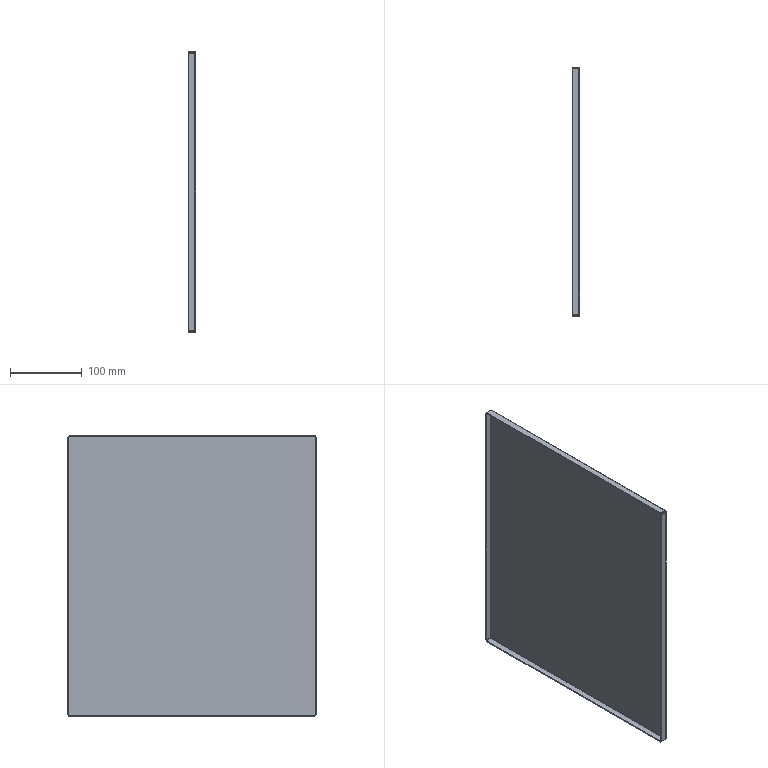Part | SolidWorks | 1 solid | 38 faces | box 10 x 346.001 x 390.001 mm | volume 220135 mm3 | plane 22 | spline 8 | cylinder 8 | commonest cylinder face diameters 0.2 x4 3.2 x4
STEP:
#1=CARTESIAN_POINT('',(-1.5,-171.4,-193.4));
#2=VERTEX_POINT('',#1);
#3=CARTESIAN_POINT('',(-1.5,171.4,-193.4));
#4=VERTEX_POINT('',#3);
#5=CARTESIAN_POINT('',(-1.5,-171.4,-193.4));
#6=DIRECTION('',(0.,1.,0.));
#7=VECTOR('',#6,1000.);
#8=LINE('',#5,#7);
#9=EDGE_CURVE('',#2,#4,#8,.T.);
#10=ORIENTED_EDGE('',*,*,#9,.F.);
#11=CARTESIAN_POINT('',(-1.5,-171.4,193.4));
#12=VERTEX_POINT('',#11);
#13=CARTESIAN_POINT('',(-1.5,-171.4,193.4));
#14=DIRECTION('',(0.,0.,-1.));
#15=VECTOR('',#14,1000.);
#16=LINE('',#13,#15);
#17=EDGE_CURVE('',#12,#2,#16,.T.);
#18=ORIENTED_EDGE('',*,*,#17,.F.);
#19=CARTESIAN_POINT('',(-1.5,171.4,193.4));
#20=VERTEX_POINT('',#19);
#21=CARTESIAN_POINT('',(-1.5,171.4,193.4));
#22=DIRECTION('',(0.,-1.,0.));
#23=VECTOR('',#22,1000.);
#24=LINE('',#21,#23);
#25=EDGE_CURVE('',#20,#12,#24,.T.);
#26=ORIENTED_EDGE('',*,*,#25,.F.);
#27=CARTESIAN_POINT('',(-1.5,171.4,-193.4));
#28=DIRECTION('',(0.,0.,1.));
#29=VECTOR('',#28,1000.);
#30=LINE('',#27,#29);
#31=EDGE_CURVE('',#4,#20,#30,.T.);
#32=ORIENTED_EDGE('',*,*,#31,.F.);
#33=EDGE_LOOP('',(#10,#18,#26,#32));
#34=FACE_OUTER_BOUND('',#33,.T.);
#35=CARTESIAN_POINT('',(-1.5,0.,0.));
#36=DIRECTION('',(1.,0.,0.));
#37=DIRECTION('',(0.,0.,-1.));
#38=AXIS2_PLACEMENT_3D('',#35,#36,#37);
#39=PLANE('',#38);
#40=ADVANCED_FACE('',(#34),#39,.F.);
#41=CARTESIAN_POINT('',(0.,-171.4,193.4));
#42=VERTEX_POINT('',#41);
#43=CARTESIAN_POINT('',(0.,-171.4,-193.4));
#44=VERTEX_POINT('',#43);
#45=CARTESIAN_POINT('',(0.,-171.4,193.4));
#46=DIRECTION('',(0.,0.,-1.));
#47=VECTOR('',#46,1000.);
#48=LINE('',#45,#47);
#49=EDGE_CURVE('',#42,#44,#48,.T.);
#50=ORIENTED_EDGE('',*,*,#49,.T.);
#51=CARTESIAN_POINT('',(0.,171.4,-193.4));
#52=VERTEX_POINT('',#51);
#53=CARTESIAN_POINT('',(0.,-171.4,-193.4));
#54=DIRECTION('',(0.,1.,0.));
#55=VECTOR('',#54,1000.);
#56=LINE('',#53,#55);
#57=EDGE_CURVE('',#44,#52,#56,.T.);
#58=ORIENTED_EDGE('',*,*,#57,.T.);
#59=CARTESIAN_POINT('',(0.,171.4,193.4));
#60=VERTEX_POINT('',#59);
#61=CARTESIAN_POINT('',(0.,171.4,-193.4));
#62=DIRECTION('',(0.,0.,1.));
#63=VECTOR('',#62,1000.);
#64=LINE('',#61,#63);
#65=EDGE_CURVE('',#52,#60,#64,.T.);
#66=ORIENTED_EDGE('',*,*,#65,.T.);
#67=CARTESIAN_POINT('',(0.,171.4,193.4));
#68=DIRECTION('',(0.,-1.,0.));
#69=VECTOR('',#68,1000.);
#70=LINE('',#67,#69);
#71=EDGE_CURVE('',#60,#42,#70,.T.);
#72=ORIENTED_EDGE('',*,*,#71,.T.);
#73=EDGE_LOOP('',(#50,#58,#66,#72));
#74=FACE_OUTER_BOUND('',#73,.T.);
#75=CARTESIAN_POINT('',(0.,0.,0.));
#76=DIRECTION('',(1.,0.,0.));
#77=DIRECTION('',(0.,0.,-1.));
#78=AXIS2_PLACEMENT_3D('',#75,#76,#77);
#79=PLANE('',#78);
#80=ADVANCED_FACE('',(#74),#79,.T.);
#81=CARTESIAN_POINT('',(-1.6,173.,192.793));
#82=VERTEX_POINT('',#81);
#83=CARTESIAN_POINT('',(-1.6,171.5,192.793));
#84=VERTEX_POINT('',#83);
#85=CARTESIAN_POINT('',(-1.6,171.5,192.793));
#86=DIRECTION('',(0.,-1.,0.));
#87=VECTOR('',#86,1000.);
#88=LINE('',#85,#87);
#89=EDGE_CURVE('',#82,#84,#88,.T.);
#90=ORIENTED_EDGE('',*,*,#89,.T.);
#91=CARTESIAN_POINT('',(-1.5,171.4,193.4));
#92=CARTESIAN_POINT('',(-1.5,171.426,193.299));
#93=CARTESIAN_POINT('',(-1.511,171.452,193.198));
#94=CARTESIAN_POINT('',(-1.548,171.489,192.995));
#95=CARTESIAN_POINT('',(-1.574,171.5,192.894));
#96=CARTESIAN_POINT('',(-1.6,171.5,192.793));
#97=B_SPLINE_CURVE_WITH_KNOTS('',3,(#91,#92,#93,#94,#95,#96),.UNSPECIFIED.,.F.,.F.,(4,2,4),(0.,0.5,1.),.UNSPECIFIED.);
#98=EDGE_CURVE('',#20,#84,#97,.T.);
#99=ORIENTED_EDGE('',*,*,#98,.F.);
#100=CARTESIAN_POINT('',(-1.5,171.4,193.4));
#101=DIRECTION('',(1.,0.,0.));
#102=VECTOR('',#101,1000.);
#103=LINE('',#100,#102);
#104=EDGE_CURVE('',#20,#60,#103,.T.);
#105=ORIENTED_EDGE('',*,*,#104,.T.);
#106=CARTESIAN_POINT('',(0.,171.4,193.4));
#107=CARTESIAN_POINT('',(0.,171.612,193.349));
#108=CARTESIAN_POINT('',(-0.04048,171.815,193.3));
#109=CARTESIAN_POINT('',(-0.2012,172.205,193.198));
#110=CARTESIAN_POINT('',(-0.3186,172.381,193.148));
#111=CARTESIAN_POINT('',(-0.5418,172.605,193.071));
#112=CARTESIAN_POINT('',(-0.6225,172.671,193.046));
#113=CARTESIAN_POINT('',(-0.7959,172.787,192.996));
#114=CARTESIAN_POINT('',(-0.8897,172.838,192.97));
#115=CARTESIAN_POINT('',(-1.18,172.958,192.894));
#116=CARTESIAN_POINT('',(-1.388,173.,192.844));
#117=CARTESIAN_POINT('',(-1.6,173.,192.793));
#118=B_SPLINE_CURVE_WITH_KNOTS('',3,(#106,#107,#108,#109,#110,#111,#112,#113,#114,#115,#116,#117),.UNSPECIFIED.,.F.,.F.,(4,2,2,2,2,4),(0.,0.0006399,0.00128,0.0016,0.00192,0.00256),.UNSPECIFIED.);
#119=EDGE_CURVE('',#60,#82,#118,.T.);
#120=ORIENTED_EDGE('',*,*,#119,.T.);
#121=EDGE_LOOP('',(#90,#99,#105,#120));
#122=FACE_OUTER_BOUND('',#121,.T.);
#123=CARTESIAN_POINT('',(0.015,171.4,193.4));
#124=CARTESIAN_POINT('',(0.015,171.611,193.349));
#125=CARTESIAN_POINT('',(-0.02703,171.823,193.299));
#126=CARTESIAN_POINT('',(-0.1888,172.213,193.198));
#127=CARTESIAN_POINT('',(-0.3085,172.392,193.147));
#128=CARTESIAN_POINT('',(-0.6075,172.691,193.046));
#129=CARTESIAN_POINT('',(-0.7867,172.811,192.995));
#130=CARTESIAN_POINT('',(-1.177,172.973,192.894));
#131=CARTESIAN_POINT('',(-1.389,173.015,192.843));
#132=CARTESIAN_POINT('',(-1.6,173.015,192.793));
#133=CARTESIAN_POINT('',(0.,171.4,193.4));
#134=CARTESIAN_POINT('',(0.,171.609,193.349));
#135=CARTESIAN_POINT('',(-0.04164,171.819,193.299));
#136=CARTESIAN_POINT('',(-0.2019,172.206,193.198));
#137=CARTESIAN_POINT('',(-0.3205,172.383,193.147));
#138=CARTESIAN_POINT('',(-0.6167,172.679,193.046));
#139=CARTESIAN_POINT('',(-0.7942,172.798,192.995));
#140=CARTESIAN_POINT('',(-1.181,172.958,192.894));
#141=CARTESIAN_POINT('',(-1.391,173.,192.843));
#142=CARTESIAN_POINT('',(-1.6,173.,192.793));
#143=CARTESIAN_POINT('',(-1.5,171.4,193.4));
#144=CARTESIAN_POINT('',(-1.5,171.413,193.349));
#145=CARTESIAN_POINT('',(-1.503,171.426,193.299));
#146=CARTESIAN_POINT('',(-1.513,171.45,193.198));
#147=CARTESIAN_POINT('',(-1.52,171.461,193.147));
#148=CARTESIAN_POINT('',(-1.539,171.48,193.046));
#149=CARTESIAN_POINT('',(-1.55,171.487,192.995));
#150=CARTESIAN_POINT('',(-1.574,171.497,192.894));
#151=CARTESIAN_POINT('',(-1.587,171.5,192.843));
#152=CARTESIAN_POINT('',(-1.6,171.5,192.793));
#153=B_SPLINE_SURFACE_WITH_KNOTS('',1,3,((#123,#124,#125,#126,#127,#128,#129,#130,#131,#132),(#133,#134,#135,#136,#137,#138,#139,#140,#141,#142),(#143,#144,#145,#146,#147,#148,#149,#150,#151,#152)),.UNSPECIFIED.,.F.,.F.,.F.,(2,1,2),(4,2,2,2,4),(-0.01,0.,1.),(0.,0.25,0.5,0.75,1.),.UNSPECIFIED.);
#154=ADVANCED_FACE('',(#122),#153,.F.);
#155=CARTESIAN_POINT('',(-1.6,171.5,-192.793));
#156=VERTEX_POINT('',#155);
#157=CARTESIAN_POINT('',(-1.6,171.5,-192.793));
#158=CARTESIAN_POINT('',(-1.574,171.5,-192.894));
#159=CARTESIAN_POINT('',(-1.548,171.489,-192.995));
#160=CARTESIAN_POINT('',(-1.511,171.452,-193.198));
#161=CARTESIAN_POINT('',(-1.5,171.426,-193.299));
#162=CARTESIAN_POINT('',(-1.5,171.4,-193.4));
#163=B_SPLINE_CURVE_WITH_KNOTS('',3,(#157,#158,#159,#160,#161,#162),.UNSPECIFIED.,.F.,.F.,(4,2,4),(0.,0.5,1.),.UNSPECIFIED.);
#164=EDGE_CURVE('',#156,#4,#163,.T.);
#165=ORIENTED_EDGE('',*,*,#164,.F.);
#166=CARTESIAN_POINT('',(-1.6,173.,-192.793));
#167=VERTEX_POINT('',#166);
#168=CARTESIAN_POINT('',(-1.6,171.5,-192.793));
#169=DIRECTION('',(0.,-1.,0.));
#170=VECTOR('',#169,1000.);
#171=LINE('',#168,#170);
#172=EDGE_CURVE('',#167,#156,#171,.T.);
#173=ORIENTED_EDGE('',*,*,#172,.F.);
#174=CARTESIAN_POINT('',(-1.6,173.,-192.793));
#175=CARTESIAN_POINT('',(-1.388,173.,-192.844));
#176=CARTESIAN_POINT('',(-1.185,172.96,-192.893));
#177=CARTESIAN_POINT('',(-0.7952,172.799,-192.995));
#178=CARTESIAN_POINT('',(-0.619,172.681,-193.045));
#179=CARTESIAN_POINT('',(-0.3953,172.458,-193.121));
#180=CARTESIAN_POINT('',(-0.329,172.378,-193.147));
#181=CARTESIAN_POINT('',(-0.2128,172.204,-193.197));
#182=CARTESIAN_POINT('',(-0.1625,172.11,-193.223));
#183=CARTESIAN_POINT('',(-0.04195,171.82,-193.299));
#184=CARTESIAN_POINT('',(0.,171.612,-193.349));
#185=CARTESIAN_POINT('',(0.,171.4,-193.4));
#186=B_SPLINE_CURVE_WITH_KNOTS('',3,(#174,#175,#176,#177,#178,#179,#180,#181,#182,#183,#184,#185),.UNSPECIFIED.,.F.,.F.,(4,2,2,2,2,4),(0.,0.0006399,0.00128,0.0016,0.00192,0.00256),.UNSPECIFIED.);
#187=EDGE_CURVE('',#167,#52,#186,.T.);
#188=ORIENTED_EDGE('',*,*,#187,.T.);
#189=CARTESIAN_POINT('',(-1.5,171.4,-193.4));
#190=DIRECTION('',(1.,0.,0.));
#191=VECTOR('',#190,1000.);
#192=LINE('',#189,#191);
#193=EDGE_CURVE('',#4,#52,#192,.T.);
#194=ORIENTED_EDGE('',*,*,#193,.F.);
#195=EDGE_LOOP('',(#165,#173,#188,#194));
#196=FACE_OUTER_BOUND('',#195,.T.);
#197=CARTESIAN_POINT('',(-1.6,173.015,-192.793));
#198=CARTESIAN_POINT('',(-1.389,173.015,-192.843));
#199=CARTESIAN_POINT('',(-1.177,172.973,-192.894));
#200=CARTESIAN_POINT('',(-0.7867,172.811,-192.995));
#201=CARTESIAN_POINT('',(-0.6075,172.691,-193.046));
#202=CARTESIAN_POINT('',(-0.3085,172.392,-193.147));
#203=CARTESIAN_POINT('',(-0.1888,172.213,-193.198));
#204=CARTESIAN_POINT('',(-0.02703,171.823,-193.299));
#205=CARTESIAN_POINT('',(0.015,171.611,-193.349));
#206=CARTESIAN_POINT('',(0.015,171.4,-193.4));
#207=CARTESIAN_POINT('',(-1.6,173.,-192.793));
#208=CARTESIAN_POINT('',(-1.391,173.,-192.843));
#209=CARTESIAN_POINT('',(-1.181,172.958,-192.894));
#210=CARTESIAN_POINT('',(-0.7942,172.798,-192.995));
#211=CARTESIAN_POINT('',(-0.6167,172.679,-193.046));
#212=CARTESIAN_POINT('',(-0.3205,172.383,-193.147));
#213=CARTESIAN_POINT('',(-0.2019,172.206,-193.198));
#214=CARTESIAN_POINT('',(-0.04164,171.819,-193.299));
#215=CARTESIAN_POINT('',(0.,171.609,-193.349));
#216=CARTESIAN_POINT('',(0.,171.4,-193.4));
#217=CARTESIAN_POINT('',(-1.6,171.5,-192.793));
#218=CARTESIAN_POINT('',(-1.587,171.5,-192.843));
#219=CARTESIAN_POINT('',(-1.574,171.497,-192.894));
#220=CARTESIAN_POINT('',(-1.55,171.487,-192.995));
#221=CARTESIAN_POINT('',(-1.539,171.48,-193.046));
#222=CARTESIAN_POINT('',(-1.52,171.461,-193.147));
#223=CARTESIAN_POINT('',(-1.513,171.45,-193.198));
#224=CARTESIAN_POINT('',(-1.503,171.426,-193.299));
#225=CARTESIAN_POINT('',(-1.5,171.413,-193.349));
#226=CARTESIAN_POINT('',(-1.5,171.4,-193.4));
#227=B_SPLINE_SURFACE_WITH_KNOTS('',1,3,((#197,#198,#199,#200,#201,#202,#203,#204,#205,#206),(#207,#208,#209,#210,#211,#212,#213,#214,#215,#216),(#217,#218,#219,#220,#221,#222,#223,#224,#225,#226)),.UNSPECIFIED.,.F.,.F.,.F.,(2,1,2),(4,2,2,2,4),(-0.01,0.,1.),(0.,0.25,0.5,0.75,1.),.UNSPECIFIED.);
#228=ADVANCED_FACE('',(#196),#227,.F.);
#229=ORIENTED_EDGE('',*,*,#65,.F.);
#230=ORIENTED_EDGE('',*,*,#187,.F.);
#231=CARTESIAN_POINT('',(-1.6,173.,0.));
#232=DIRECTION('',(0.,0.,-1.));
#233=VECTOR('',#232,1000.);
#234=LINE('',#231,#233);
#235=EDGE_CURVE('',#82,#167,#234,.T.);
#236=ORIENTED_EDGE('',*,*,#235,.F.);
#237=ORIENTED_EDGE('',*,*,#119,.F.);
#238=EDGE_LOOP('',(#229,#230,#236,#237));
#239=FACE_OUTER_BOUND('',#238,.T.);
#240=CARTESIAN_POINT('',(-1.6,171.4,-193.4));
#241=DIRECTION('',(0.,0.,-1.));
#242=DIRECTION('',(0.,1.,0.));
#243=AXIS2_PLACEMENT_3D('',#240,#241,#242);
#244=CYLINDRICAL_SURFACE('',#243,1.6);
#245=ADVANCED_FACE('',(#239),#244,.T.);
#246=ORIENTED_EDGE('',*,*,#31,.T.);
#247=ORIENTED_EDGE('',*,*,#98,.T.);
#248=CARTESIAN_POINT('',(-1.6,171.5,195.));
#249=DIRECTION('',(0.,0.,-1.));
#250=VECTOR('',#249,1000.);
#251=LINE('',#248,#250);
#252=EDGE_CURVE('',#84,#156,#251,.T.);
#253=ORIENTED_EDGE('',*,*,#252,.T.);
#254=ORIENTED_EDGE('',*,*,#164,.T.);
#255=EDGE_LOOP('',(#246,#247,#253,#254));
#256=FACE_OUTER_BOUND('',#255,.T.);
#257=CARTESIAN_POINT('',(-1.6,171.4,-193.4));
#258=DIRECTION('',(0.,0.,-1.));
#259=DIRECTION('',(0.,1.,0.));
#260=AXIS2_PLACEMENT_3D('',#257,#258,#259);
#261=CYLINDRICAL_SURFACE('',#260,0.1);
#262=ADVANCED_FACE('',(#256),#261,.F.);
#263=CARTESIAN_POINT('',(-10.,171.5,192.793));
#264=VERTEX_POINT('',#263);
#265=CARTESIAN_POINT('',(-10.,173.,192.793));
#266=VERTEX_POINT('',#265);
#267=CARTESIAN_POINT('',(-10.,173.,192.793));
#268=DIRECTION('',(0.,1.,0.));
#269=VECTOR('',#268,1000.);
#270=LINE('',#267,#269);
#271=EDGE_CURVE('',#264,#266,#270,.T.);
#272=ORIENTED_EDGE('',*,*,#271,.F.);
#273=CARTESIAN_POINT('',(0.,171.5,192.793));
#274=DIRECTION('',(-1.,0.,0.));
#275=VECTOR('',#274,1000.);
#276=LINE('',#273,#275);
#277=EDGE_CURVE('',#84,#264,#276,.T.);
#278=ORIENTED_EDGE('',*,*,#277,.F.);
#279=ORIENTED_EDGE('',*,*,#89,.F.);
#280=CARTESIAN_POINT('',(0.,173.,192.793));
#281=DIRECTION('',(1.,0.,0.));
#282=VECTOR('',#281,1000.);
#283=LINE('',#280,#282);
#284=EDGE_CURVE('',#266,#82,#283,.T.);
#285=ORIENTED_EDGE('',*,*,#284,.F.);
#286=EDGE_LOOP('',(#272,#278,#279,#285));
#287=FACE_OUTER_BOUND('',#286,.T.);
#288=CARTESIAN_POINT('',(-1.5,171.5,192.793));
#289=DIRECTION('',(0.,0.,1.));
#290=DIRECTION('',(1.,0.,0.));
#291=AXIS2_PLACEMENT_3D('',#288,#289,#290);
#292=PLANE('',#291);
#293=ADVANCED_FACE('',(#287),#292,.T.);
#294=CARTESIAN_POINT('',(-10.,173.,-192.793));
#295=VERTEX_POINT('',#294);
#296=CARTESIAN_POINT('',(-1.5,173.,-192.793));
#297=DIRECTION('',(1.,0.,0.));
#298=VECTOR('',#297,1000.);
#299=LINE('',#296,#298);
#300=EDGE_CURVE('',#295,#167,#299,.T.);
#301=ORIENTED_EDGE('',*,*,#300,.F.);
#302=CARTESIAN_POINT('',(-10.,173.,-195.));
#303=DIRECTION('',(0.,0.,-1.));
#304=VECTOR('',#303,1000.);
#305=LINE('',#302,#304);
#306=EDGE_CURVE('',#266,#295,#305,.T.);
#307=ORIENTED_EDGE('',*,*,#306,.F.);
#308=ORIENTED_EDGE('',*,*,#284,.T.);
#309=ORIENTED_EDGE('',*,*,#235,.T.);
#310=EDGE_LOOP('',(#301,#307,#308,#309));
#311=FACE_OUTER_BOUND('',#310,.T.);
#312=CARTESIAN_POINT('',(0.,173.,0.));
#313=DIRECTION('',(0.,1.,0.));
#314=DIRECTION('',(-1.,0.,0.));
#315=AXIS2_PLACEMENT_3D('',#312,#313,#314);
#316=PLANE('',#315);
#317=ADVANCED_FACE('',(#311),#316,.T.);
#318=CARTESIAN_POINT('',(-10.,171.5,-192.793));
#319=VERTEX_POINT('',#318);
#320=CARTESIAN_POINT('',(-10.,171.5,0.));
#321=DIRECTION('',(0.,0.,-1.));
#322=VECTOR('',#321,1000.);
#323=LINE('',#320,#322);
#324=EDGE_CURVE('',#264,#319,#323,.T.);
#325=ORIENTED_EDGE('',*,*,#324,.T.);
#326=CARTESIAN_POINT('',(-1.5,171.5,-192.793));
#327=DIRECTION('',(-1.,0.,0.));
#328=VECTOR('',#327,1000.);
#329=LINE('',#326,#328);
#330=EDGE_CURVE('',#156,#319,#329,.T.);
#331=ORIENTED_EDGE('',*,*,#330,.F.);
#332=ORIENTED_EDGE('',*,*,#252,.F.);
#333=ORIENTED_EDGE('',*,*,#277,.T.);
#334=EDGE_LOOP('',(#325,#331,#332,#333));
#335=FACE_OUTER_BOUND('',#334,.T.);
#336=CARTESIAN_POINT('',(0.,171.5,0.));
#337=DIRECTION('',(0.,1.,0.));
#338=DIRECTION('',(-1.,0.,0.));
#339=AXIS2_PLACEMENT_3D('',#336,#337,#338);
#340=PLANE('',#339);
#341=ADVANCED_FACE('',(#335),#340,.F.);
#342=CARTESIAN_POINT('',(-10.,171.5,-192.793));
#343=DIRECTION('',(0.,1.,0.));
#344=VECTOR('',#343,1000.);
#345=LINE('',#342,#344);
#346=EDGE_CURVE('',#319,#295,#345,.T.);
#347=ORIENTED_EDGE('',*,*,#346,.F.);
#348=ORIENTED_EDGE('',*,*,#324,.F.);
#349=ORIENTED_EDGE('',*,*,#271,.T.);
#350=ORIENTED_EDGE('',*,*,#306,.T.);
#351=EDGE_LOOP('',(#347,#348,#349,#350));
#352=FACE_OUTER_BOUND('',#351,.T.);
#353=CARTESIAN_POINT('',(-10.,173.,-195.));
#354=DIRECTION('',(-1.,0.,0.));
#355=DIRECTION('',(0.,-1.,0.));
#356=AXIS2_PLACEMENT_3D('',#353,#354,#355);
#357=PLANE('',#356);
#358=ADVANCED_FACE('',(#352),#357,.T.);
#359=ORIENTED_EDGE('',*,*,#330,.T.);
#360=ORIENTED_EDGE('',*,*,#346,.T.);
#361=ORIENTED_EDGE('',*,*,#300,.T.);
#362=ORIENTED_EDGE('',*,*,#172,.T.);
#363=EDGE_LOOP('',(#359,#360,#361,#362));
#364=FACE_OUTER_BOUND('',#363,.T.);
#365=CARTESIAN_POINT('',(-1.5,171.5,-192.793));
#366=DIRECTION('',(0.,0.,1.));
#367=DIRECTION('',(1.,0.,0.));
#368=AXIS2_PLACEMENT_3D('',#365,#366,#367);
#369=PLANE('',#368);
#370=ADVANCED_FACE('',(#364),#369,.F.);
#371=CARTESIAN_POINT('',(-1.6,-170.793,195.));
#372=VERTEX_POINT('',#371);
#373=CARTESIAN_POINT('',(-1.6,-170.793,193.5));
#374=VERTEX_POINT('',#373);
#375=CARTESIAN_POINT('',(-1.6,-170.793,193.5));
#376=DIRECTION('',(0.,0.,-1.));
#377=VECTOR('',#376,1000.);
#378=LINE('',#375,#377);
#379=EDGE_CURVE('',#372,#374,#378,.T.);
#380=ORIENTED_EDGE('',*,*,#379,.T.);
#381=CARTESIAN_POINT('',(-1.5,-171.4,193.4));
#382=CARTESIAN_POINT('',(-1.5,-171.299,193.426));
#383=CARTESIAN_POINT('',(-1.511,-171.198,193.452));
#384=CARTESIAN_POINT('',(-1.548,-170.995,193.489));
#385=CARTESIAN_POINT('',(-1.574,-170.894,193.5));
#386=CARTESIAN_POINT('',(-1.6,-170.793,193.5));
#387=B_SPLINE_CURVE_WITH_KNOTS('',3,(#381,#382,#383,#384,#385,#386),.UNSPECIFIED.,.F.,.F.,(4,2,4),(0.,0.5,1.),.UNSPECIFIED.);
#388=EDGE_CURVE('',#12,#374,#387,.T.);
#389=ORIENTED_EDGE('',*,*,#388,.F.);
#390=CARTESIAN_POINT('',(-1.5,-171.4,193.4));
#391=DIRECTION('',(1.,0.,0.));
#392=VECTOR('',#391,1000.);
#393=LINE('',#390,#392);
#394=EDGE_CURVE('',#12,#42,#393,.T.);
#395=ORIENTED_EDGE('',*,*,#394,.T.);
#396=CARTESIAN_POINT('',(0.,-171.4,193.4));
#397=CARTESIAN_POINT('',(0.,-171.349,193.612));
#398=CARTESIAN_POINT('',(-0.04048,-171.3,193.815));
#399=CARTESIAN_POINT('',(-0.2012,-171.198,194.205));
#400=CARTESIAN_POINT('',(-0.3186,-171.148,194.381));
#401=CARTESIAN_POINT('',(-0.5418,-171.071,194.605));
#402=CARTESIAN_POINT('',(-0.6225,-171.046,194.671));
#403=CARTESIAN_POINT('',(-0.7959,-170.996,194.787));
#404=CARTESIAN_POINT('',(-0.8897,-170.97,194.838));
#405=CARTESIAN_POINT('',(-1.18,-170.894,194.958));
#406=CARTESIAN_POINT('',(-1.388,-170.844,195.));
#407=CARTESIAN_POINT('',(-1.6,-170.793,195.));
#408=B_SPLINE_CURVE_WITH_KNOTS('',3,(#396,#397,#398,#399,#400,#401,#402,#403,#404,#405,#406,#407),.UNSPECIFIED.,.F.,.F.,(4,2,2,2,2,4),(0.,0.0006399,0.00128,0.0016,0.00192,0.00256),.UNSPECIFIED.);
#409=EDGE_CURVE('',#42,#372,#408,.T.);
#410=ORIENTED_EDGE('',*,*,#409,.T.);
#411=EDGE_LOOP('',(#380,#389,#395,#410));
#412=FACE_OUTER_BOUND('',#411,.T.);
#413=CARTESIAN_POINT('',(0.015,-171.4,193.4));
#414=CARTESIAN_POINT('',(0.015,-171.349,193.611));
#415=CARTESIAN_POINT('',(-0.02703,-171.299,193.823));
#416=CARTESIAN_POINT('',(-0.1888,-171.198,194.213));
#417=CARTESIAN_POINT('',(-0.3085,-171.147,194.392));
#418=CARTESIAN_POINT('',(-0.6075,-171.046,194.691));
#419=CARTESIAN_POINT('',(-0.7867,-170.995,194.811));
#420=CARTESIAN_POINT('',(-1.177,-170.894,194.973));
#421=CARTESIAN_POINT('',(-1.389,-170.843,195.015));
#422=CARTESIAN_POINT('',(-1.6,-170.793,195.015));
#423=CARTESIAN_POINT('',(0.,-171.4,193.4));
#424=CARTESIAN_POINT('',(0.,-171.349,193.609));
#425=CARTESIAN_POINT('',(-0.04164,-171.299,193.819));
#426=CARTESIAN_POINT('',(-0.2019,-171.198,194.206));
#427=CARTESIAN_POINT('',(-0.3205,-171.147,194.383));
#428=CARTESIAN_POINT('',(-0.6167,-171.046,194.679));
#429=CARTESIAN_POINT('',(-0.7942,-170.995,194.798));
#430=CARTESIAN_POINT('',(-1.181,-170.894,194.958));
#431=CARTESIAN_POINT('',(-1.391,-170.843,195.));
#432=CARTESIAN_POINT('',(-1.6,-170.793,195.));
#433=CARTESIAN_POINT('',(-1.5,-171.4,193.4));
#434=CARTESIAN_POINT('',(-1.5,-171.349,193.413));
#435=CARTESIAN_POINT('',(-1.503,-171.299,193.426));
#436=CARTESIAN_POINT('',(-1.513,-171.198,193.45));
#437=CARTESIAN_POINT('',(-1.52,-171.147,193.461));
#438=CARTESIAN_POINT('',(-1.539,-171.046,193.48));
#439=CARTESIAN_POINT('',(-1.55,-170.995,193.487));
#440=CARTESIAN_POINT('',(-1.574,-170.894,193.497));
#441=CARTESIAN_POINT('',(-1.587,-170.843,193.5));
#442=CARTESIAN_POINT('',(-1.6,-170.793,193.5));
#443=B_SPLINE_SURFACE_WITH_KNOTS('',1,3,((#413,#414,#415,#416,#417,#418,#419,#420,#421,#422),(#423,#424,#425,#426,#427,#428,#429,#430,#431,#432),(#433,#434,#435,#436,#437,#438,#439,#440,#441,#442)),.UNSPECIFIED.,.F.,.F.,.F.,(2,1,2),(4,2,2,2,4),(-0.01,0.,1.),(0.,0.25,0.5,0.75,1.),.UNSPECIFIED.);
#444=ADVANCED_FACE('',(#412),#443,.F.);
#445=CARTESIAN_POINT('',(-1.6,170.793,193.5));
#446=VERTEX_POINT('',#445);
#447=CARTESIAN_POINT('',(-1.6,170.793,193.5));
#448=CARTESIAN_POINT('',(-1.574,170.894,193.5));
#449=CARTESIAN_POINT('',(-1.548,170.995,193.489));
#450=CARTESIAN_POINT('',(-1.511,171.198,193.452));
#451=CARTESIAN_POINT('',(-1.5,171.299,193.426));
#452=CARTESIAN_POINT('',(-1.5,171.4,193.4));
#453=B_SPLINE_CURVE_WITH_KNOTS('',3,(#447,#448,#449,#450,#451,#452),.UNSPECIFIED.,.F.,.F.,(4,2,4),(0.,0.5,1.),.UNSPECIFIED.);
#454=EDGE_CURVE('',#446,#20,#453,.T.);
#455=ORIENTED_EDGE('',*,*,#454,.F.);
#456=CARTESIAN_POINT('',(-1.6,170.793,195.));
#457=VERTEX_POINT('',#456);
#458=CARTESIAN_POINT('',(-1.6,170.793,193.5));
#459=DIRECTION('',(0.,0.,-1.));
#460=VECTOR('',#459,1000.);
#461=LINE('',#458,#460);
#462=EDGE_CURVE('',#457,#446,#461,.T.);
#463=ORIENTED_EDGE('',*,*,#462,.F.);
#464=CARTESIAN_POINT('',(-1.6,170.793,195.));
#465=CARTESIAN_POINT('',(-1.388,170.844,195.));
#466=CARTESIAN_POINT('',(-1.185,170.893,194.96));
#467=CARTESIAN_POINT('',(-0.7952,170.995,194.799));
#468=CARTESIAN_POINT('',(-0.619,171.045,194.681));
#469=CARTESIAN_POINT('',(-0.3953,171.121,194.458));
#470=CARTESIAN_POINT('',(-0.329,171.147,194.378));
#471=CARTESIAN_POINT('',(-0.2128,171.197,194.204));
#472=CARTESIAN_POINT('',(-0.1625,171.223,194.11));
#473=CARTESIAN_POINT('',(-0.04195,171.299,193.82));
#474=CARTESIAN_POINT('',(0.,171.349,193.612));
#475=CARTESIAN_POINT('',(0.,171.4,193.4));
#476=B_SPLINE_CURVE_WITH_KNOTS('',3,(#464,#465,#466,#467,#468,#469,#470,#471,#472,#473,#474,#475),.UNSPECIFIED.,.F.,.F.,(4,2,2,2,2,4),(0.,0.0006399,0.00128,0.0016,0.00192,0.00256),.UNSPECIFIED.);
#477=EDGE_CURVE('',#457,#60,#476,.T.);
#478=ORIENTED_EDGE('',*,*,#477,.T.);
#479=ORIENTED_EDGE('',*,*,#104,.F.);
#480=EDGE_LOOP('',(#455,#463,#478,#479));
#481=FACE_OUTER_BOUND('',#480,.T.);
#482=CARTESIAN_POINT('',(-1.6,170.793,195.015));
#483=CARTESIAN_POINT('',(-1.389,170.843,195.015));
#484=CARTESIAN_POINT('',(-1.177,170.894,194.973));
#485=CARTESIAN_POINT('',(-0.7867,170.995,194.811));
#486=CARTESIAN_POINT('',(-0.6075,171.046,194.691));
#487=CARTESIAN_POINT('',(-0.3085,171.147,194.392));
#488=CARTESIAN_POINT('',(-0.1888,171.198,194.213));
#489=CARTESIAN_POINT('',(-0.02703,171.299,193.823));
#490=CARTESIAN_POINT('',(0.015,171.349,193.611));
#491=CARTESIAN_POINT('',(0.015,171.4,193.4));
#492=CARTESIAN_POINT('',(-1.6,170.793,195.));
#493=CARTESIAN_POINT('',(-1.391,170.843,195.));
#494=CARTESIAN_POINT('',(-1.181,170.894,194.958));
#495=CARTESIAN_POINT('',(-0.7942,170.995,194.798));
#496=CARTESIAN_POINT('',(-0.6167,171.046,194.679));
#497=CARTESIAN_POINT('',(-0.3205,171.147,194.383));
#498=CARTESIAN_POINT('',(-0.2019,171.198,194.206));
#499=CARTESIAN_POINT('',(-0.04164,171.299,193.819));
#500=CARTESIAN_POINT('',(0.,171.349,193.609));
#501=CARTESIAN_POINT('',(0.,171.4,193.4));
#502=CARTESIAN_POINT('',(-1.6,170.793,193.5));
#503=CARTESIAN_POINT('',(-1.587,170.843,193.5));
#504=CARTESIAN_POINT('',(-1.574,170.894,193.497));
#505=CARTESIAN_POINT('',(-1.55,170.995,193.487));
#506=CARTESIAN_POINT('',(-1.539,171.046,193.48));
#507=CARTESIAN_POINT('',(-1.52,171.147,193.461));
#508=CARTESIAN_POINT('',(-1.513,171.198,193.45));
#509=CARTESIAN_POINT('',(-1.503,171.299,193.426));
#510=CARTESIAN_POINT('',(-1.5,171.349,193.413));
#511=CARTESIAN_POINT('',(-1.5,171.4,193.4));
#512=B_SPLINE_SURFACE_WITH_KNOTS('',1,3,((#482,#483,#484,#485,#486,#487,#488,#489,#490,#491),(#492,#493,#494,#495,#496,#497,#498,#499,#500,#501),(#502,#503,#504,#505,#506,#507,#508,#509,#510,#511)),.UNSPECIFIED.,.F.,.F.,.F.,(2,1,2),(4,2,2,2,4),(-0.01,0.,1.),(0.,0.25,0.5,0.75,1.),.UNSPECIFIED.);
#513=ADVANCED_FACE('',(#481),#512,.F.);
#514=ORIENTED_EDGE('',*,*,#71,.F.);
#515=ORIENTED_EDGE('',*,*,#477,.F.);
#516=CARTESIAN_POINT('',(-1.6,-173.,195.));
#517=DIRECTION('',(0.,-1.,0.));
#518=VECTOR('',#517,1000.);
#519=LINE('',#516,#518);
#520=EDGE_CURVE('',#457,#372,#519,.T.);
#521=ORIENTED_EDGE('',*,*,#520,.T.);
#522=ORIENTED_EDGE('',*,*,#409,.F.);
#523=EDGE_LOOP('',(#514,#515,#521,#522));
#524=FACE_OUTER_BOUND('',#523,.T.);
#525=CARTESIAN_POINT('',(-1.6,171.4,193.4));
#526=DIRECTION('',(0.,1.,0.));
#527=DIRECTION('',(0.,0.,1.));
#528=AXIS2_PLACEMENT_3D('',#525,#526,#527);
#529=CYLINDRICAL_SURFACE('',#528,1.6);
#530=ADVANCED_FACE('',(#524),#529,.T.);
#531=ORIENTED_EDGE('',*,*,#25,.T.);
#532=ORIENTED_EDGE('',*,*,#388,.T.);
#533=CARTESIAN_POINT('',(-1.6,-173.,193.5));
#534=DIRECTION('',(0.,1.,0.));
#535=VECTOR('',#534,1000.);
#536=LINE('',#533,#535);
#537=EDGE_CURVE('',#374,#446,#536,.T.);
#538=ORIENTED_EDGE('',*,*,#537,.T.);
#539=ORIENTED_EDGE('',*,*,#454,.T.);
#540=EDGE_LOOP('',(#531,#532,#538,#539));
#541=FACE_OUTER_BOUND('',#540,.T.);
#542=CARTESIAN_POINT('',(-1.6,171.4,193.4));
#543=DIRECTION('',(0.,1.,0.));
#544=DIRECTION('',(0.,0.,1.));
#545=AXIS2_PLACEMENT_3D('',#542,#543,#544);
#546=CYLINDRICAL_SURFACE('',#545,0.1);
#547=ADVANCED_FACE('',(#541),#546,.F.);
#548=CARTESIAN_POINT('',(-10.,-170.793,193.5));
#549=VERTEX_POINT('',#548);
#550=CARTESIAN_POINT('',(-10.,-170.793,195.));
#551=VERTEX_POINT('',#550);
#552=CARTESIAN_POINT('',(-10.,-170.793,195.));
#553=DIRECTION('',(0.,0.,1.));
#554=VECTOR('',#553,1000.);
#555=LINE('',#552,#554);
#556=EDGE_CURVE('',#549,#551,#555,.T.);
#557=ORIENTED_EDGE('',*,*,#556,.F.);
#558=CARTESIAN_POINT('',(0.,-170.793,193.5));
#559=DIRECTION('',(-1.,0.,0.));
#560=VECTOR('',#559,1000.);
#561=LINE('',#558,#560);
#562=EDGE_CURVE('',#374,#549,#561,.T.);
#563=ORIENTED_EDGE('',*,*,#562,.F.);
#564=ORIENTED_EDGE('',*,*,#379,.F.);
#565=CARTESIAN_POINT('',(-1.5,-170.793,195.));
#566=DIRECTION('',(-1.,0.,0.));
#567=VECTOR('',#566,1000.);
#568=LINE('',#565,#567);
#569=EDGE_CURVE('',#372,#551,#568,.T.);
#570=ORIENTED_EDGE('',*,*,#569,.T.);
#571=EDGE_LOOP('',(#557,#563,#564,#570));
#572=FACE_OUTER_BOUND('',#571,.T.);
#573=CARTESIAN_POINT('',(-1.5,-170.793,193.5));
#574=DIRECTION('',(0.,-1.,0.));
#575=DIRECTION('',(0.,0.,-1.));
#576=AXIS2_PLACEMENT_3D('',#573,#574,#575);
#577=PLANE('',#576);
#578=ADVANCED_FACE('',(#572),#577,.T.);
#579=ORIENTED_EDGE('',*,*,#520,.F.);
#580=CARTESIAN_POINT('',(-10.,170.793,195.));
#581=VERTEX_POINT('',#580);
#582=CARTESIAN_POINT('',(0.,170.793,195.));
#583=DIRECTION('',(-1.,0.,0.));
#584=VECTOR('',#583,1000.);
#585=LINE('',#582,#584);
#586=EDGE_CURVE('',#457,#581,#585,.T.);
#587=ORIENTED_EDGE('',*,*,#586,.T.);
#588=CARTESIAN_POINT('',(-10.,-173.,195.));
#589=DIRECTION('',(0.,1.,0.));
#590=VECTOR('',#589,1000.);
#591=LINE('',#588,#590);
#592=EDGE_CURVE('',#551,#581,#591,.T.);
#593=ORIENTED_EDGE('',*,*,#592,.F.);
#594=ORIENTED_EDGE('',*,*,#569,.F.);
#595=EDGE_LOOP('',(#579,#587,#593,#594));
#596=FACE_OUTER_BOUND('',#595,.T.);
#597=CARTESIAN_POINT('',(0.,0.,195.));
#598=DIRECTION('',(0.,0.,-1.));
#599=DIRECTION('',(-1.,0.,0.));
#600=AXIS2_PLACEMENT_3D('',#597,#598,#599);
#601=PLANE('',#600);
#602=ADVANCED_FACE('',(#596),#601,.F.);
#603=CARTESIAN_POINT('',(-10.,170.793,193.5));
#604=VERTEX_POINT('',#603);
#605=CARTESIAN_POINT('',(-1.5,170.793,193.5));
#606=DIRECTION('',(-1.,0.,0.));
#607=VECTOR('',#606,1000.);
#608=LINE('',#605,#607);
#609=EDGE_CURVE('',#446,#604,#608,.T.);
#610=ORIENTED_EDGE('',*,*,#609,.F.);
#611=ORIENTED_EDGE('',*,*,#537,.F.);
#612=ORIENTED_EDGE('',*,*,#562,.T.);
#613=CARTESIAN_POINT('',(-10.,0.,193.5));
#614=DIRECTION('',(0.,1.,0.));
#615=VECTOR('',#614,1000.);
#616=LINE('',#613,#615);
#617=EDGE_CURVE('',#549,#604,#616,.T.);
#618=ORIENTED_EDGE('',*,*,#617,.T.);
#619=EDGE_LOOP('',(#610,#611,#612,#618));
#620=FACE_OUTER_BOUND('',#619,.T.);
#621=CARTESIAN_POINT('',(0.,0.,193.5));
#622=DIRECTION('',(0.,0.,-1.));
#623=DIRECTION('',(-1.,0.,0.));
#624=AXIS2_PLACEMENT_3D('',#621,#622,#623);
#625=PLANE('',#624);
#626=ADVANCED_FACE('',(#620),#625,.T.);
#627=CARTESIAN_POINT('',(-10.,170.793,193.5));
#628=DIRECTION('',(0.,0.,1.));
#629=VECTOR('',#628,1000.);
#630=LINE('',#627,#629);
#631=EDGE_CURVE('',#604,#581,#630,.T.);
#632=ORIENTED_EDGE('',*,*,#631,.F.);
#633=ORIENTED_EDGE('',*,*,#617,.F.);
#634=ORIENTED_EDGE('',*,*,#556,.T.);
#635=ORIENTED_EDGE('',*,*,#592,.T.);
#636=EDGE_LOOP('',(#632,#633,#634,#635));
#637=FACE_OUTER_BOUND('',#636,.T.);
#638=CARTESIAN_POINT('',(-10.,-173.,195.));
#639=DIRECTION('',(-1.,0.,0.));
#640=DIRECTION('',(0.,0.,1.));
#641=AXIS2_PLACEMENT_3D('',#638,#639,#640);
#642=PLANE('',#641);
#643=ADVANCED_FACE('',(#637),#642,.T.);
#644=ORIENTED_EDGE('',*,*,#609,.T.);
#645=ORIENTED_EDGE('',*,*,#631,.T.);
#646=ORIENTED_EDGE('',*,*,#586,.F.);
#647=ORIENTED_EDGE('',*,*,#462,.T.);
#648=EDGE_LOOP('',(#644,#645,#646,#647));
#649=FACE_OUTER_BOUND('',#648,.T.);
#650=CARTESIAN_POINT('',(-1.5,170.793,193.5));
#651=DIRECTION('',(0.,-1.,0.));
#652=DIRECTION('',(0.,0.,-1.));
#653=AXIS2_PLACEMENT_3D('',#650,#651,#652);
#654=PLANE('',#653);
#655=ADVANCED_FACE('',(#649),#654,.F.);
#656=CARTESIAN_POINT('',(-1.6,-173.,-192.793));
#657=VERTEX_POINT('',#656);
#658=CARTESIAN_POINT('',(-1.6,-171.5,-192.793));
#659=VERTEX_POINT('',#658);
#660=CARTESIAN_POINT('',(-1.6,-171.5,-192.793));
#661=DIRECTION('',(0.,1.,0.));
#662=VECTOR('',#661,1000.);
#663=LINE('',#660,#662);
#664=EDGE_CURVE('',#657,#659,#663,.T.);
#665=ORIENTED_EDGE('',*,*,#664,.T.);
#666=CARTESIAN_POINT('',(-1.5,-171.4,-193.4));
#667=CARTESIAN_POINT('',(-1.5,-171.426,-193.299));
#668=CARTESIAN_POINT('',(-1.511,-171.452,-193.198));
#669=CARTESIAN_POINT('',(-1.548,-171.489,-192.995));
#670=CARTESIAN_POINT('',(-1.574,-171.5,-192.894));
#671=CARTESIAN_POINT('',(-1.6,-171.5,-192.793));
#672=B_SPLINE_CURVE_WITH_KNOTS('',3,(#666,#667,#668,#669,#670,#671),.UNSPECIFIED.,.F.,.F.,(4,2,4),(0.,0.5,1.),.UNSPECIFIED.);
#673=EDGE_CURVE('',#2,#659,#672,.T.);
#674=ORIENTED_EDGE('',*,*,#673,.F.);
#675=CARTESIAN_POINT('',(-1.5,-171.4,-193.4));
#676=DIRECTION('',(1.,0.,0.));
#677=VECTOR('',#676,1000.);
#678=LINE('',#675,#677);
#679=EDGE_CURVE('',#2,#44,#678,.T.);
#680=ORIENTED_EDGE('',*,*,#679,.T.);
#681=CARTESIAN_POINT('',(0.,-171.4,-193.4));
#682=CARTESIAN_POINT('',(0.,-171.612,-193.349));
#683=CARTESIAN_POINT('',(-0.04048,-171.815,-193.3));
#684=CARTESIAN_POINT('',(-0.2012,-172.205,-193.198));
#685=CARTESIAN_POINT('',(-0.3186,-172.381,-193.148));
#686=CARTESIAN_POINT('',(-0.5418,-172.605,-193.071));
#687=CARTESIAN_POINT('',(-0.6225,-172.671,-193.046));
#688=CARTESIAN_POINT('',(-0.7959,-172.787,-192.996));
#689=CARTESIAN_POINT('',(-0.8897,-172.838,-192.97));
#690=CARTESIAN_POINT('',(-1.18,-172.958,-192.894));
#691=CARTESIAN_POINT('',(-1.388,-173.,-192.844));
#692=CARTESIAN_POINT('',(-1.6,-173.,-192.793));
#693=B_SPLINE_CURVE_WITH_KNOTS('',3,(#681,#682,#683,#684,#685,#686,#687,#688,#689,#690,#691,#692),.UNSPECIFIED.,.F.,.F.,(4,2,2,2,2,4),(0.,0.0006399,0.00128,0.0016,0.00192,0.00256),.UNSPECIFIED.);
#694=EDGE_CURVE('',#44,#657,#693,.T.);
#695=ORIENTED_EDGE('',*,*,#694,.T.);
#696=EDGE_LOOP('',(#665,#674,#680,#695));
#697=FACE_OUTER_BOUND('',#696,.T.);
#698=CARTESIAN_POINT('',(0.015,-171.4,-193.4));
#699=CARTESIAN_POINT('',(0.015,-171.611,-193.349));
#700=CARTESIAN_POINT('',(-0.02703,-171.823,-193.299));
#701=CARTESIAN_POINT('',(-0.1888,-172.213,-193.198));
#702=CARTESIAN_POINT('',(-0.3085,-172.392,-193.147));
#703=CARTESIAN_POINT('',(-0.6075,-172.691,-193.046));
#704=CARTESIAN_POINT('',(-0.7867,-172.811,-192.995));
#705=CARTESIAN_POINT('',(-1.177,-172.973,-192.894));
#706=CARTESIAN_POINT('',(-1.389,-173.015,-192.843));
#707=CARTESIAN_POINT('',(-1.6,-173.015,-192.793));
#708=CARTESIAN_POINT('',(0.,-171.4,-193.4));
#709=CARTESIAN_POINT('',(0.,-171.609,-193.349));
#710=CARTESIAN_POINT('',(-0.04164,-171.819,-193.299));
#711=CARTESIAN_POINT('',(-0.2019,-172.206,-193.198));
#712=CARTESIAN_POINT('',(-0.3205,-172.383,-193.147));
#713=CARTESIAN_POINT('',(-0.6167,-172.679,-193.046));
#714=CARTESIAN_POINT('',(-0.7942,-172.798,-192.995));
#715=CARTESIAN_POINT('',(-1.181,-172.958,-192.894));
#716=CARTESIAN_POINT('',(-1.391,-173.,-192.843));
#717=CARTESIAN_POINT('',(-1.6,-173.,-192.793));
#718=CARTESIAN_POINT('',(-1.5,-171.4,-193.4));
#719=CARTESIAN_POINT('',(-1.5,-171.413,-193.349));
#720=CARTESIAN_POINT('',(-1.503,-171.426,-193.299));
#721=CARTESIAN_POINT('',(-1.513,-171.45,-193.198));
#722=CARTESIAN_POINT('',(-1.52,-171.461,-193.147));
#723=CARTESIAN_POINT('',(-1.539,-171.48,-193.046));
#724=CARTESIAN_POINT('',(-1.55,-171.487,-192.995));
#725=CARTESIAN_POINT('',(-1.574,-171.497,-192.894));
#726=CARTESIAN_POINT('',(-1.587,-171.5,-192.843));
#727=CARTESIAN_POINT('',(-1.6,-171.5,-192.793));
#728=B_SPLINE_SURFACE_WITH_KNOTS('',1,3,((#698,#699,#700,#701,#702,#703,#704,#705,#706,#707),(#708,#709,#710,#711,#712,#713,#714,#715,#716,#717),(#718,#719,#720,#721,#722,#723,#724,#725,#726,#727)),.UNSPECIFIED.,.F.,.F.,.F.,(2,1,2),(4,2,2,2,4),(-0.01,0.,1.),(0.,0.25,0.5,0.75,1.),.UNSPECIFIED.);
#729=ADVANCED_FACE('',(#697),#728,.F.);
#730=CARTESIAN_POINT('',(-1.6,-171.5,192.793));
#731=VERTEX_POINT('',#730);
#732=CARTESIAN_POINT('',(-1.6,-171.5,192.793));
#733=CARTESIAN_POINT('',(-1.574,-171.5,192.894));
#734=CARTESIAN_POINT('',(-1.548,-171.489,192.995));
#735=CARTESIAN_POINT('',(-1.511,-171.452,193.198));
#736=CARTESIAN_POINT('',(-1.5,-171.426,193.299));
#737=CARTESIAN_POINT('',(-1.5,-171.4,193.4));
#738=B_SPLINE_CURVE_WITH_KNOTS('',3,(#732,#733,#734,#735,#736,#737),.UNSPECIFIED.,.F.,.F.,(4,2,4),(0.,0.5,1.),.UNSPECIFIED.);
#739=EDGE_CURVE('',#731,#12,#738,.T.);
#740=ORIENTED_EDGE('',*,*,#739,.F.);
#741=CARTESIAN_POINT('',(-1.6,-173.,192.793));
#742=VERTEX_POINT('',#741);
#743=CARTESIAN_POINT('',(-1.6,-171.5,192.793));
#744=DIRECTION('',(0.,1.,0.));
#745=VECTOR('',#744,1000.);
#746=LINE('',#743,#745);
#747=EDGE_CURVE('',#742,#731,#746,.T.);
#748=ORIENTED_EDGE('',*,*,#747,.F.);
#749=CARTESIAN_POINT('',(-1.6,-173.,192.793));
#750=CARTESIAN_POINT('',(-1.388,-173.,192.844));
#751=CARTESIAN_POINT('',(-1.185,-172.96,192.893));
#752=CARTESIAN_POINT('',(-0.7952,-172.799,192.995));
#753=CARTESIAN_POINT('',(-0.619,-172.681,193.045));
#754=CARTESIAN_POINT('',(-0.3953,-172.458,193.121));
#755=CARTESIAN_POINT('',(-0.329,-172.378,193.147));
#756=CARTESIAN_POINT('',(-0.2128,-172.204,193.197));
#757=CARTESIAN_POINT('',(-0.1625,-172.11,193.223));
#758=CARTESIAN_POINT('',(-0.04195,-171.82,193.299));
#759=CARTESIAN_POINT('',(0.,-171.612,193.349));
#760=CARTESIAN_POINT('',(0.,-171.4,193.4));
#761=B_SPLINE_CURVE_WITH_KNOTS('',3,(#749,#750,#751,#752,#753,#754,#755,#756,#757,#758,#759,#760),.UNSPECIFIED.,.F.,.F.,(4,2,2,2,2,4),(0.,0.0006399,0.00128,0.0016,0.00192,0.00256),.UNSPECIFIED.);
#762=EDGE_CURVE('',#742,#42,#761,.T.);
#763=ORIENTED_EDGE('',*,*,#762,.T.);
#764=ORIENTED_EDGE('',*,*,#394,.F.);
#765=EDGE_LOOP('',(#740,#748,#763,#764));
#766=FACE_OUTER_BOUND('',#765,.T.);
#767=CARTESIAN_POINT('',(-1.6,-173.015,192.793));
#768=CARTESIAN_POINT('',(-1.389,-173.015,192.843));
#769=CARTESIAN_POINT('',(-1.177,-172.973,192.894));
#770=CARTESIAN_POINT('',(-0.7867,-172.811,192.995));
#771=CARTESIAN_POINT('',(-0.6075,-172.691,193.046));
#772=CARTESIAN_POINT('',(-0.3085,-172.392,193.147));
#773=CARTESIAN_POINT('',(-0.1888,-172.213,193.198));
#774=CARTESIAN_POINT('',(-0.02703,-171.823,193.299));
#775=CARTESIAN_POINT('',(0.015,-171.611,193.349));
#776=CARTESIAN_POINT('',(0.015,-171.4,193.4));
#777=CARTESIAN_POINT('',(-1.6,-173.,192.793));
#778=CARTESIAN_POINT('',(-1.391,-173.,192.843));
#779=CARTESIAN_POINT('',(-1.181,-172.958,192.894));
#780=CARTESIAN_POINT('',(-0.7942,-172.798,192.995));
#781=CARTESIAN_POINT('',(-0.6167,-172.679,193.046));
#782=CARTESIAN_POINT('',(-0.3205,-172.383,193.147));
#783=CARTESIAN_POINT('',(-0.2019,-172.206,193.198));
#784=CARTESIAN_POINT('',(-0.04164,-171.819,193.299));
#785=CARTESIAN_POINT('',(0.,-171.609,193.349));
#786=CARTESIAN_POINT('',(0.,-171.4,193.4));
#787=CARTESIAN_POINT('',(-1.6,-171.5,192.793));
#788=CARTESIAN_POINT('',(-1.587,-171.5,192.843));
#789=CARTESIAN_POINT('',(-1.574,-171.497,192.894));
#790=CARTESIAN_POINT('',(-1.55,-171.487,192.995));
#791=CARTESIAN_POINT('',(-1.539,-171.48,193.046));
#792=CARTESIAN_POINT('',(-1.52,-171.461,193.147));
#793=CARTESIAN_POINT('',(-1.513,-171.45,193.198));
#794=CARTESIAN_POINT('',(-1.503,-171.426,193.299));
#795=CARTESIAN_POINT('',(-1.5,-171.413,193.349));
#796=CARTESIAN_POINT('',(-1.5,-171.4,193.4));
#797=B_SPLINE_SURFACE_WITH_KNOTS('',1,3,((#767,#768,#769,#770,#771,#772,#773,#774,#775,#776),(#777,#778,#779,#780,#781,#782,#783,#784,#785,#786),(#787,#788,#789,#790,#791,#792,#793,#794,#795,#796)),.UNSPECIFIED.,.F.,.F.,.F.,(2,1,2),(4,2,2,2,4),(-0.01,0.,1.),(0.,0.25,0.5,0.75,1.),.UNSPECIFIED.);
#798=ADVANCED_FACE('',(#766),#797,.F.);
#799=ORIENTED_EDGE('',*,*,#49,.F.);
#800=ORIENTED_EDGE('',*,*,#762,.F.);
#801=CARTESIAN_POINT('',(-1.6,-173.,-195.));
#802=DIRECTION('',(0.,0.,-1.));
#803=VECTOR('',#802,1000.);
#804=LINE('',#801,#803);
#805=EDGE_CURVE('',#742,#657,#804,.T.);
#806=ORIENTED_EDGE('',*,*,#805,.T.);
#807=ORIENTED_EDGE('',*,*,#694,.F.);
#808=EDGE_LOOP('',(#799,#800,#806,#807));
#809=FACE_OUTER_BOUND('',#808,.T.);
#810=CARTESIAN_POINT('',(-1.6,-171.4,193.4));
#811=DIRECTION('',(0.,0.,1.));
#812=DIRECTION('',(0.,-1.,0.));
#813=AXIS2_PLACEMENT_3D('',#810,#811,#812);
#814=CYLINDRICAL_SURFACE('',#813,1.6);
#815=ADVANCED_FACE('',(#809),#814,.T.);
#816=ORIENTED_EDGE('',*,*,#17,.T.);
#817=ORIENTED_EDGE('',*,*,#673,.T.);
#818=CARTESIAN_POINT('',(-1.6,-171.5,-195.));
#819=DIRECTION('',(0.,0.,1.));
#820=VECTOR('',#819,1000.);
#821=LINE('',#818,#820);
#822=EDGE_CURVE('',#659,#731,#821,.T.);
#823=ORIENTED_EDGE('',*,*,#822,.T.);
#824=ORIENTED_EDGE('',*,*,#739,.T.);
#825=EDGE_LOOP('',(#816,#817,#823,#824));
#826=FACE_OUTER_BOUND('',#825,.T.);
#827=CARTESIAN_POINT('',(-1.6,-171.4,193.4));
#828=DIRECTION('',(0.,0.,1.));
#829=DIRECTION('',(0.,-1.,0.));
#830=AXIS2_PLACEMENT_3D('',#827,#828,#829);
#831=CYLINDRICAL_SURFACE('',#830,0.1);
#832=ADVANCED_FACE('',(#826),#831,.F.);
#833=CARTESIAN_POINT('',(-10.,-171.5,-192.793));
#834=VERTEX_POINT('',#833);
#835=CARTESIAN_POINT('',(-10.,-173.,-192.793));
#836=VERTEX_POINT('',#835);
#837=CARTESIAN_POINT('',(-10.,-173.,-192.793));
#838=DIRECTION('',(0.,-1.,0.));
#839=VECTOR('',#838,1000.);
#840=LINE('',#837,#839);
#841=EDGE_CURVE('',#834,#836,#840,.T.);
#842=ORIENTED_EDGE('',*,*,#841,.F.);
#843=CARTESIAN_POINT('',(0.,-171.5,-192.793));
#844=DIRECTION('',(-1.,0.,0.));
#845=VECTOR('',#844,1000.);
#846=LINE('',#843,#845);
#847=EDGE_CURVE('',#659,#834,#846,.T.);
#848=ORIENTED_EDGE('',*,*,#847,.F.);
#849=ORIENTED_EDGE('',*,*,#664,.F.);
#850=CARTESIAN_POINT('',(-1.5,-173.,-192.793));
#851=DIRECTION('',(-1.,0.,0.));
#852=VECTOR('',#851,1000.);
#853=LINE('',#850,#852);
#854=EDGE_CURVE('',#657,#836,#853,.T.);
#855=ORIENTED_EDGE('',*,*,#854,.T.);
#856=EDGE_LOOP('',(#842,#848,#849,#855));
#857=FACE_OUTER_BOUND('',#856,.T.);
#858=CARTESIAN_POINT('',(-1.5,-171.5,-192.793));
#859=DIRECTION('',(0.,0.,-1.));
#860=DIRECTION('',(-1.,0.,0.));
#861=AXIS2_PLACEMENT_3D('',#858,#859,#860);
#862=PLANE('',#861);
#863=ADVANCED_FACE('',(#857),#862,.T.);
#864=ORIENTED_EDGE('',*,*,#805,.F.);
#865=CARTESIAN_POINT('',(-10.,-173.,192.793));
#866=VERTEX_POINT('',#865);
#867=CARTESIAN_POINT('',(0.,-173.,192.793));
#868=DIRECTION('',(-1.,0.,0.));
#869=VECTOR('',#868,1000.);
#870=LINE('',#867,#869);
#871=EDGE_CURVE('',#742,#866,#870,.T.);
#872=ORIENTED_EDGE('',*,*,#871,.T.);
#873=CARTESIAN_POINT('',(-10.,-173.,-195.));
#874=DIRECTION('',(0.,0.,1.));
#875=VECTOR('',#874,1000.);
#876=LINE('',#873,#875);
#877=EDGE_CURVE('',#836,#866,#876,.T.);
#878=ORIENTED_EDGE('',*,*,#877,.F.);
#879=ORIENTED_EDGE('',*,*,#854,.F.);
#880=EDGE_LOOP('',(#864,#872,#878,#879));
#881=FACE_OUTER_BOUND('',#880,.T.);
#882=CARTESIAN_POINT('',(0.,-173.,0.));
#883=DIRECTION('',(0.,1.,0.));
#884=DIRECTION('',(-1.,0.,0.));
#885=AXIS2_PLACEMENT_3D('',#882,#883,#884);
#886=PLANE('',#885);
#887=ADVANCED_FACE('',(#881),#886,.F.);
#888=CARTESIAN_POINT('',(-10.,-171.5,192.793));
#889=VERTEX_POINT('',#888);
#890=CARTESIAN_POINT('',(-1.5,-171.5,192.793));
#891=DIRECTION('',(-1.,0.,0.));
#892=VECTOR('',#891,1000.);
#893=LINE('',#890,#892);
#894=EDGE_CURVE('',#731,#889,#893,.T.);
#895=ORIENTED_EDGE('',*,*,#894,.F.);
#896=ORIENTED_EDGE('',*,*,#822,.F.);
#897=ORIENTED_EDGE('',*,*,#847,.T.);
#898=CARTESIAN_POINT('',(-10.,-171.5,0.));
#899=DIRECTION('',(0.,0.,1.));
#900=VECTOR('',#899,1000.);
#901=LINE('',#898,#900);
#902=EDGE_CURVE('',#834,#889,#901,.T.);
#903=ORIENTED_EDGE('',*,*,#902,.T.);
#904=EDGE_LOOP('',(#895,#896,#897,#903));
#905=FACE_OUTER_BOUND('',#904,.T.);
#906=CARTESIAN_POINT('',(0.,-171.5,0.));
#907=DIRECTION('',(0.,1.,0.));
#908=DIRECTION('',(-1.,0.,0.));
#909=AXIS2_PLACEMENT_3D('',#906,#907,#908);
#910=PLANE('',#909);
#911=ADVANCED_FACE('',(#905),#910,.T.);
#912=CARTESIAN_POINT('',(-10.,-171.5,192.793));
#913=DIRECTION('',(0.,-1.,0.));
#914=VECTOR('',#913,1000.);
#915=LINE('',#912,#914);
#916=EDGE_CURVE('',#889,#866,#915,.T.);
#917=ORIENTED_EDGE('',*,*,#916,.F.);
#918=ORIENTED_EDGE('',*,*,#902,.F.);
#919=ORIENTED_EDGE('',*,*,#841,.T.);
#920=ORIENTED_EDGE('',*,*,#877,.T.);
#921=EDGE_LOOP('',(#917,#918,#919,#920));
#922=FACE_OUTER_BOUND('',#921,.T.);
#923=CARTESIAN_POINT('',(-10.,-173.,-195.));
#924=DIRECTION('',(-1.,0.,0.));
#925=DIRECTION('',(0.,-1.,0.));
#926=AXIS2_PLACEMENT_3D('',#923,#924,#925);
#927=PLANE('',#926);
#928=ADVANCED_FACE('',(#922),#927,.T.);
#929=ORIENTED_EDGE('',*,*,#894,.T.);
#930=ORIENTED_EDGE('',*,*,#916,.T.);
#931=ORIENTED_EDGE('',*,*,#871,.F.);
#932=ORIENTED_EDGE('',*,*,#747,.T.);
#933=EDGE_LOOP('',(#929,#930,#931,#932));
#934=FACE_OUTER_BOUND('',#933,.T.);
#935=CARTESIAN_POINT('',(-1.5,-171.5,192.793));
#936=DIRECTION('',(0.,0.,-1.));
#937=DIRECTION('',(-1.,0.,0.));
#938=AXIS2_PLACEMENT_3D('',#935,#936,#937);
#939=PLANE('',#938);
#940=ADVANCED_FACE('',(#934),#939,.F.);
#941=CARTESIAN_POINT('',(-1.6,170.793,-195.));
#942=VERTEX_POINT('',#941);
#943=CARTESIAN_POINT('',(-1.6,170.793,-193.5));
#944=VERTEX_POINT('',#943);
#945=CARTESIAN_POINT('',(-1.6,170.793,-193.5));
#946=DIRECTION('',(0.,0.,1.));
#947=VECTOR('',#946,1000.);
#948=LINE('',#945,#947);
#949=EDGE_CURVE('',#942,#944,#948,.T.);
#950=ORIENTED_EDGE('',*,*,#949,.T.);
#951=CARTESIAN_POINT('',(-1.5,171.4,-193.4));
#952=CARTESIAN_POINT('',(-1.5,171.299,-193.426));
#953=CARTESIAN_POINT('',(-1.511,171.198,-193.452));
#954=CARTESIAN_POINT('',(-1.548,170.995,-193.489));
#955=CARTESIAN_POINT('',(-1.574,170.894,-193.5));
#956=CARTESIAN_POINT('',(-1.6,170.793,-193.5));
#957=B_SPLINE_CURVE_WITH_KNOTS('',3,(#951,#952,#953,#954,#955,#956),.UNSPECIFIED.,.F.,.F.,(4,2,4),(0.,0.5,1.),.UNSPECIFIED.);
#958=EDGE_CURVE('',#4,#944,#957,.T.);
#959=ORIENTED_EDGE('',*,*,#958,.F.);
#960=ORIENTED_EDGE('',*,*,#193,.T.);
#961=CARTESIAN_POINT('',(0.,171.4,-193.4));
#962=CARTESIAN_POINT('',(0.,171.349,-193.612));
#963=CARTESIAN_POINT('',(-0.04048,171.3,-193.815));
#964=CARTESIAN_POINT('',(-0.2012,171.198,-194.205));
#965=CARTESIAN_POINT('',(-0.3186,171.148,-194.381));
#966=CARTESIAN_POINT('',(-0.5418,171.071,-194.605));
#967=CARTESIAN_POINT('',(-0.6225,171.046,-194.671));
#968=CARTESIAN_POINT('',(-0.7959,170.996,-194.787));
#969=CARTESIAN_POINT('',(-0.8897,170.97,-194.838));
#970=CARTESIAN_POINT('',(-1.18,170.894,-194.958));
#971=CARTESIAN_POINT('',(-1.388,170.844,-195.));
#972=CARTESIAN_POINT('',(-1.6,170.793,-195.));
#973=B_SPLINE_CURVE_WITH_KNOTS('',3,(#961,#962,#963,#964,#965,#966,#967,#968,#969,#970,#971,#972),.UNSPECIFIED.,.F.,.F.,(4,2,2,2,2,4),(0.,0.0006399,0.00128,0.0016,0.00192,0.00256),.UNSPECIFIED.);
#974=EDGE_CURVE('',#52,#942,#973,.T.);
#975=ORIENTED_EDGE('',*,*,#974,.T.);
#976=EDGE_LOOP('',(#950,#959,#960,#975));
#977=FACE_OUTER_BOUND('',#976,.T.);
#978=CARTESIAN_POINT('',(0.015,171.4,-193.4));
#979=CARTESIAN_POINT('',(0.015,171.349,-193.611));
#980=CARTESIAN_POINT('',(-0.02703,171.299,-193.823));
#981=CARTESIAN_POINT('',(-0.1888,171.198,-194.213));
#982=CARTESIAN_POINT('',(-0.3085,171.147,-194.392));
#983=CARTESIAN_POINT('',(-0.6075,171.046,-194.691));
#984=CARTESIAN_POINT('',(-0.7867,170.995,-194.811));
#985=CARTESIAN_POINT('',(-1.177,170.894,-194.973));
#986=CARTESIAN_POINT('',(-1.389,170.843,-195.015));
#987=CARTESIAN_POINT('',(-1.6,170.793,-195.015));
#988=CARTESIAN_POINT('',(0.,171.4,-193.4));
#989=CARTESIAN_POINT('',(0.,171.349,-193.609));
#990=CARTESIAN_POINT('',(-0.04164,171.299,-193.819));
#991=CARTESIAN_POINT('',(-0.2019,171.198,-194.206));
#992=CARTESIAN_POINT('',(-0.3205,171.147,-194.383));
#993=CARTESIAN_POINT('',(-0.6167,171.046,-194.679));
#994=CARTESIAN_POINT('',(-0.7942,170.995,-194.798));
#995=CARTESIAN_POINT('',(-1.181,170.894,-194.958));
#996=CARTESIAN_POINT('',(-1.391,170.843,-195.));
#997=CARTESIAN_POINT('',(-1.6,170.793,-195.));
#998=CARTESIAN_POINT('',(-1.5,171.4,-193.4));
#999=CARTESIAN_POINT('',(-1.5,171.349,-193.413));
#1000=CARTESIAN_POINT('',(-1.503,171.299,-193.426));
#1001=CARTESIAN_POINT('',(-1.513,171.198,-193.45));
#1002=CARTESIAN_POINT('',(-1.52,171.147,-193.461));
#1003=CARTESIAN_POINT('',(-1.539,171.046,-193.48));
#1004=CARTESIAN_POINT('',(-1.55,170.995,-193.487));
#1005=CARTESIAN_POINT('',(-1.574,170.894,-193.497));
#1006=CARTESIAN_POINT('',(-1.587,170.843,-193.5));
#1007=CARTESIAN_POINT('',(-1.6,170.793,-193.5));
#1008=B_SPLINE_SURFACE_WITH_KNOTS('',1,3,((#978,#979,#980,#981,#982,#983,#984,#985,#986,#987),(#988,#989,#990,#991,#992,#993,#994,#995,#996,#997),(#998,#999,#1000,#1001,#1002,#1003,#1004,#1005,#1006,#1007)),.UNSPECIFIED.,.F.,.F.,.F.,(2,1,2),(4,2,2,2,4),(-0.01,0.,1.),(0.,0.25,0.5,0.75,1.),.UNSPECIFIED.);
#1009=ADVANCED_FACE('',(#977),#1008,.F.);
#1010=CARTESIAN_POINT('',(-1.6,-170.793,-193.5));
#1011=VERTEX_POINT('',#1010);
#1012=CARTESIAN_POINT('',(-1.6,-170.793,-193.5));
#1013=CARTESIAN_POINT('',(-1.574,-170.894,-193.5));
#1014=CARTESIAN_POINT('',(-1.548,-170.995,-193.489));
#1015=CARTESIAN_POINT('',(-1.511,-171.198,-193.452));
#1016=CARTESIAN_POINT('',(-1.5,-171.299,-193.426));
#1017=CARTESIAN_POINT('',(-1.5,-171.4,-193.4));
#1018=B_SPLINE_CURVE_WITH_KNOTS('',3,(#1012,#1013,#1014,#1015,#1016,#1017),.UNSPECIFIED.,.F.,.F.,(4,2,4),(0.,0.5,1.),.UNSPECIFIED.);
#1019=EDGE_CURVE('',#1011,#2,#1018,.T.);
#1020=ORIENTED_EDGE('',*,*,#1019,.F.);
#1021=CARTESIAN_POINT('',(-1.6,-170.793,-195.));
#1022=VERTEX_POINT('',#1021);
#1023=CARTESIAN_POINT('',(-1.6,-170.793,-193.5));
#1024=DIRECTION('',(0.,0.,1.));
#1025=VECTOR('',#1024,1000.);
#1026=LINE('',#1023,#1025);
#1027=EDGE_CURVE('',#1022,#1011,#1026,.T.);
#1028=ORIENTED_EDGE('',*,*,#1027,.F.);
#1029=CARTESIAN_POINT('',(-1.6,-170.793,-195.));
#1030=CARTESIAN_POINT('',(-1.388,-170.844,-195.));
#1031=CARTESIAN_POINT('',(-1.185,-170.893,-194.96));
#1032=CARTESIAN_POINT('',(-0.7952,-170.995,-194.799));
#1033=CARTESIAN_POINT('',(-0.619,-171.045,-194.681));
#1034=CARTESIAN_POINT('',(-0.3953,-171.121,-194.458));
#1035=CARTESIAN_POINT('',(-0.329,-171.147,-194.378));
#1036=CARTESIAN_POINT('',(-0.2128,-171.197,-194.204));
#1037=CARTESIAN_POINT('',(-0.1625,-171.223,-194.11));
#1038=CARTESIAN_POINT('',(-0.04195,-171.299,-193.82));
#1039=CARTESIAN_POINT('',(0.,-171.349,-193.612));
#1040=CARTESIAN_POINT('',(0.,-171.4,-193.4));
#1041=B_SPLINE_CURVE_WITH_KNOTS('',3,(#1029,#1030,#1031,#1032,#1033,#1034,#1035,#1036,#1037,#1038,#1039,#1040),.UNSPECIFIED.,.F.,.F.,(4,2,2,2,2,4),(0.,0.0006399,0.00128,0.0016,0.00192,0.00256),.UNSPECIFIED.);
#1042=EDGE_CURVE('',#1022,#44,#1041,.T.);
#1043=ORIENTED_EDGE('',*,*,#1042,.T.);
#1044=ORIENTED_EDGE('',*,*,#679,.F.);
#1045=EDGE_LOOP('',(#1020,#1028,#1043,#1044));
#1046=FACE_OUTER_BOUND('',#1045,.T.);
#1047=CARTESIAN_POINT('',(-1.6,-170.793,-195.015));
#1048=CARTESIAN_POINT('',(-1.389,-170.843,-195.015));
#1049=CARTESIAN_POINT('',(-1.177,-170.894,-194.973));
#1050=CARTESIAN_POINT('',(-0.7867,-170.995,-194.811));
#1051=CARTESIAN_POINT('',(-0.6075,-171.046,-194.691));
#1052=CARTESIAN_POINT('',(-0.3085,-171.147,-194.392));
#1053=CARTESIAN_POINT('',(-0.1888,-171.198,-194.213));
#1054=CARTESIAN_POINT('',(-0.02703,-171.299,-193.823));
#1055=CARTESIAN_POINT('',(0.015,-171.349,-193.611));
#1056=CARTESIAN_POINT('',(0.015,-171.4,-193.4));
#1057=CARTESIAN_POINT('',(-1.6,-170.793,-195.));
#1058=CARTESIAN_POINT('',(-1.391,-170.843,-195.));
#1059=CARTESIAN_POINT('',(-1.181,-170.894,-194.958));
#1060=CARTESIAN_POINT('',(-0.7942,-170.995,-194.798));
#1061=CARTESIAN_POINT('',(-0.6167,-171.046,-194.679));
#1062=CARTESIAN_POINT('',(-0.3205,-171.147,-194.383));
#1063=CARTESIAN_POINT('',(-0.2019,-171.198,-194.206));
#1064=CARTESIAN_POINT('',(-0.04164,-171.299,-193.819));
#1065=CARTESIAN_POINT('',(0.,-171.349,-193.609));
#1066=CARTESIAN_POINT('',(0.,-171.4,-193.4));
#1067=CARTESIAN_POINT('',(-1.6,-170.793,-193.5));
#1068=CARTESIAN_POINT('',(-1.587,-170.843,-193.5));
#1069=CARTESIAN_POINT('',(-1.574,-170.894,-193.497));
#1070=CARTESIAN_POINT('',(-1.55,-170.995,-193.487));
#1071=CARTESIAN_POINT('',(-1.539,-171.046,-193.48));
#1072=CARTESIAN_POINT('',(-1.52,-171.147,-193.461));
#1073=CARTESIAN_POINT('',(-1.513,-171.198,-193.45));
#1074=CARTESIAN_POINT('',(-1.503,-171.299,-193.426));
#1075=CARTESIAN_POINT('',(-1.5,-171.349,-193.413));
#1076=CARTESIAN_POINT('',(-1.5,-171.4,-193.4));
#1077=B_SPLINE_SURFACE_WITH_KNOTS('',1,3,((#1047,#1048,#1049,#1050,#1051,#1052,#1053,#1054,#1055,#1056),(#1057,#1058,#1059,#1060,#1061,#1062,#1063,#1064,#1065,#1066),(#1067,#1068,#1069,#1070,#1071,#1072,#1073,#1074,#1075,#1076)),.UNSPECIFIED.,.F.,.F.,.F.,(2,1,2),(4,2,2,2,4),(-0.01,0.,1.),(0.,0.25,0.5,0.75,1.),.UNSPECIFIED.);
#1078=ADVANCED_FACE('',(#1046),#1077,.F.);
#1079=ORIENTED_EDGE('',*,*,#57,.F.);
#1080=ORIENTED_EDGE('',*,*,#1042,.F.);
#1081=CARTESIAN_POINT('',(-1.6,173.,-195.));
#1082=DIRECTION('',(0.,1.,0.));
#1083=VECTOR('',#1082,1000.);
#1084=LINE('',#1081,#1083);
#1085=EDGE_CURVE('',#1022,#942,#1084,.T.);
#1086=ORIENTED_EDGE('',*,*,#1085,.T.);
#1087=ORIENTED_EDGE('',*,*,#974,.F.);
#1088=EDGE_LOOP('',(#1079,#1080,#1086,#1087));
#1089=FACE_OUTER_BOUND('',#1088,.T.);
#1090=CARTESIAN_POINT('',(-1.6,-171.4,-193.4));
#1091=DIRECTION('',(0.,-1.,0.));
#1092=DIRECTION('',(0.,0.,-1.));
#1093=AXIS2_PLACEMENT_3D('',#1090,#1091,#1092);
#1094=CYLINDRICAL_SURFACE('',#1093,1.6);
#1095=ADVANCED_FACE('',(#1089),#1094,.T.);
#1096=ORIENTED_EDGE('',*,*,#9,.T.);
#1097=ORIENTED_EDGE('',*,*,#958,.T.);
#1098=CARTESIAN_POINT('',(-1.6,173.,-193.5));
#1099=DIRECTION('',(0.,-1.,0.));
#1100=VECTOR('',#1099,1000.);
#1101=LINE('',#1098,#1100);
#1102=EDGE_CURVE('',#944,#1011,#1101,.T.);
#1103=ORIENTED_EDGE('',*,*,#1102,.T.);
#1104=ORIENTED_EDGE('',*,*,#1019,.T.);
#1105=EDGE_LOOP('',(#1096,#1097,#1103,#1104));
#1106=FACE_OUTER_BOUND('',#1105,.T.);
#1107=CARTESIAN_POINT('',(-1.6,-171.4,-193.4));
#1108=DIRECTION('',(0.,-1.,0.));
#1109=DIRECTION('',(0.,0.,-1.));
#1110=AXIS2_PLACEMENT_3D('',#1107,#1108,#1109);
#1111=CYLINDRICAL_SURFACE('',#1110,0.1);
#1112=ADVANCED_FACE('',(#1106),#1111,.F.);
#1113=CARTESIAN_POINT('',(-10.,170.793,-193.5));
#1114=VERTEX_POINT('',#1113);
#1115=CARTESIAN_POINT('',(-10.,170.793,-195.));
#1116=VERTEX_POINT('',#1115);
#1117=CARTESIAN_POINT('',(-10.,170.793,-195.));
#1118=DIRECTION('',(0.,0.,-1.));
#1119=VECTOR('',#1118,1000.);
#1120=LINE('',#1117,#1119);
#1121=EDGE_CURVE('',#1114,#1116,#1120,.T.);
#1122=ORIENTED_EDGE('',*,*,#1121,.F.);
#1123=CARTESIAN_POINT('',(0.,170.793,-193.5));
#1124=DIRECTION('',(-1.,0.,0.));
#1125=VECTOR('',#1124,1000.);
#1126=LINE('',#1123,#1125);
#1127=EDGE_CURVE('',#944,#1114,#1126,.T.);
#1128=ORIENTED_EDGE('',*,*,#1127,.F.);
#1129=ORIENTED_EDGE('',*,*,#949,.F.);
#1130=CARTESIAN_POINT('',(-1.5,170.793,-195.));
#1131=DIRECTION('',(-1.,0.,0.));
#1132=VECTOR('',#1131,1000.);
#1133=LINE('',#1130,#1132);
#1134=EDGE_CURVE('',#942,#1116,#1133,.T.);
#1135=ORIENTED_EDGE('',*,*,#1134,.T.);
#1136=EDGE_LOOP('',(#1122,#1128,#1129,#1135));
#1137=FACE_OUTER_BOUND('',#1136,.T.);
#1138=CARTESIAN_POINT('',(-1.5,170.793,-193.5));
#1139=DIRECTION('',(0.,1.,0.));
#1140=DIRECTION('',(0.,0.,1.));
#1141=AXIS2_PLACEMENT_3D('',#1138,#1139,#1140);
#1142=PLANE('',#1141);
#1143=ADVANCED_FACE('',(#1137),#1142,.T.);
#1144=ORIENTED_EDGE('',*,*,#1085,.F.);
#1145=CARTESIAN_POINT('',(-10.,-170.793,-195.));
#1146=VERTEX_POINT('',#1145);
#1147=CARTESIAN_POINT('',(0.,-170.793,-195.));
#1148=DIRECTION('',(-1.,0.,0.));
#1149=VECTOR('',#1148,1000.);
#1150=LINE('',#1147,#1149);
#1151=EDGE_CURVE('',#1022,#1146,#1150,.T.);
#1152=ORIENTED_EDGE('',*,*,#1151,.T.);
#1153=CARTESIAN_POINT('',(-10.,173.,-195.));
#1154=DIRECTION('',(0.,-1.,0.));
#1155=VECTOR('',#1154,1000.);
#1156=LINE('',#1153,#1155);
#1157=EDGE_CURVE('',#1116,#1146,#1156,.T.);
#1158=ORIENTED_EDGE('',*,*,#1157,.F.);
#1159=ORIENTED_EDGE('',*,*,#1134,.F.);
#1160=EDGE_LOOP('',(#1144,#1152,#1158,#1159));
#1161=FACE_OUTER_BOUND('',#1160,.T.);
#1162=CARTESIAN_POINT('',(0.,0.,-195.));
#1163=DIRECTION('',(0.,0.,1.));
#1164=DIRECTION('',(1.,0.,0.));
#1165=AXIS2_PLACEMENT_3D('',#1162,#1163,#1164);
#1166=PLANE('',#1165);
#1167=ADVANCED_FACE('',(#1161),#1166,.F.);
#1168=CARTESIAN_POINT('',(-10.,-170.793,-193.5));
#1169=VERTEX_POINT('',#1168);
#1170=CARTESIAN_POINT('',(-1.5,-170.793,-193.5));
#1171=DIRECTION('',(-1.,0.,0.));
#1172=VECTOR('',#1171,1000.);
#1173=LINE('',#1170,#1172);
#1174=EDGE_CURVE('',#1011,#1169,#1173,.T.);
#1175=ORIENTED_EDGE('',*,*,#1174,.F.);
#1176=ORIENTED_EDGE('',*,*,#1102,.F.);
#1177=ORIENTED_EDGE('',*,*,#1127,.T.);
#1178=CARTESIAN_POINT('',(-10.,0.,-193.5));
#1179=DIRECTION('',(0.,-1.,0.));
#1180=VECTOR('',#1179,1000.);
#1181=LINE('',#1178,#1180);
#1182=EDGE_CURVE('',#1114,#1169,#1181,.T.);
#1183=ORIENTED_EDGE('',*,*,#1182,.T.);
#1184=EDGE_LOOP('',(#1175,#1176,#1177,#1183));
#1185=FACE_OUTER_BOUND('',#1184,.T.);
#1186=CARTESIAN_POINT('',(0.,0.,-193.5));
#1187=DIRECTION('',(0.,0.,1.));
#1188=DIRECTION('',(1.,0.,0.));
#1189=AXIS2_PLACEMENT_3D('',#1186,#1187,#1188);
#1190=PLANE('',#1189);
#1191=ADVANCED_FACE('',(#1185),#1190,.T.);
#1192=CARTESIAN_POINT('',(-10.,-170.793,-193.5));
#1193=DIRECTION('',(0.,0.,-1.));
#1194=VECTOR('',#1193,1000.);
#1195=LINE('',#1192,#1194);
#1196=EDGE_CURVE('',#1169,#1146,#1195,.T.);
#1197=ORIENTED_EDGE('',*,*,#1196,.F.);
#1198=ORIENTED_EDGE('',*,*,#1182,.F.);
#1199=ORIENTED_EDGE('',*,*,#1121,.T.);
#1200=ORIENTED_EDGE('',*,*,#1157,.T.);
#1201=EDGE_LOOP('',(#1197,#1198,#1199,#1200));
#1202=FACE_OUTER_BOUND('',#1201,.T.);
#1203=CARTESIAN_POINT('',(-10.,173.,-195.));
#1204=DIRECTION('',(-1.,0.,0.));
#1205=DIRECTION('',(0.,0.,1.));
#1206=AXIS2_PLACEMENT_3D('',#1203,#1204,#1205);
#1207=PLANE('',#1206);
#1208=ADVANCED_FACE('',(#1202),#1207,.T.);
#1209=ORIENTED_EDGE('',*,*,#1174,.T.);
#1210=ORIENTED_EDGE('',*,*,#1196,.T.);
#1211=ORIENTED_EDGE('',*,*,#1151,.F.);
#1212=ORIENTED_EDGE('',*,*,#1027,.T.);
#1213=EDGE_LOOP('',(#1209,#1210,#1211,#1212));
#1214=FACE_OUTER_BOUND('',#1213,.T.);
#1215=CARTESIAN_POINT('',(-1.5,-170.793,-193.5));
#1216=DIRECTION('',(0.,1.,0.));
#1217=DIRECTION('',(0.,0.,1.));
#1218=AXIS2_PLACEMENT_3D('',#1215,#1216,#1217);
#1219=PLANE('',#1218);
#1220=ADVANCED_FACE('',(#1214),#1219,.F.);
#1221=CLOSED_SHELL('',(#40,#80,#154,#228,#245,#262,#293,#317,#341,#358,#370,#444,#513,#530,#547,#578,#602,#626,#643,#655,#729,#798,#815,#832,#863,#887,#911,#928,#940,#1009,#1078,#1095,#1112,#1143,#1167,#1191,#1208,#1220));
#1222=MANIFOLD_SOLID_BREP('',#1221);
#1223=CARTESIAN_POINT('',(0.,0.,0.));
#1224=DIRECTION('',(0.,0.,1.));
#1225=DIRECTION('',(1.,0.,0.));
#1226=AXIS2_PLACEMENT_3D('',#1223,#1224,#1225);
#1227=(LENGTH_UNIT()NAMED_UNIT(*)SI_UNIT(.MILLI.,.METRE.));
#1228=UNCERTAINTY_MEASURE_WITH_UNIT(LENGTH_MEASURE(0.00001),#1227,'','');
#1229=(NAMED_UNIT(*)PLANE_ANGLE_UNIT()SI_UNIT($,.RADIAN.));
#1230=(NAMED_UNIT(*)SI_UNIT($,.STERADIAN.)SOLID_ANGLE_UNIT());
#1231=(GEOMETRIC_REPRESENTATION_CONTEXT(3)GLOBAL_UNCERTAINTY_ASSIGNED_CONTEXT((#1228))GLOBAL_UNIT_ASSIGNED_CONTEXT((#1227,#1229,#1230))REPRESENTATION_CONTEXT('',''));
#1232=ADVANCED_BREP_SHAPE_REPRESENTATION('',(#1222,#1226),#1231);